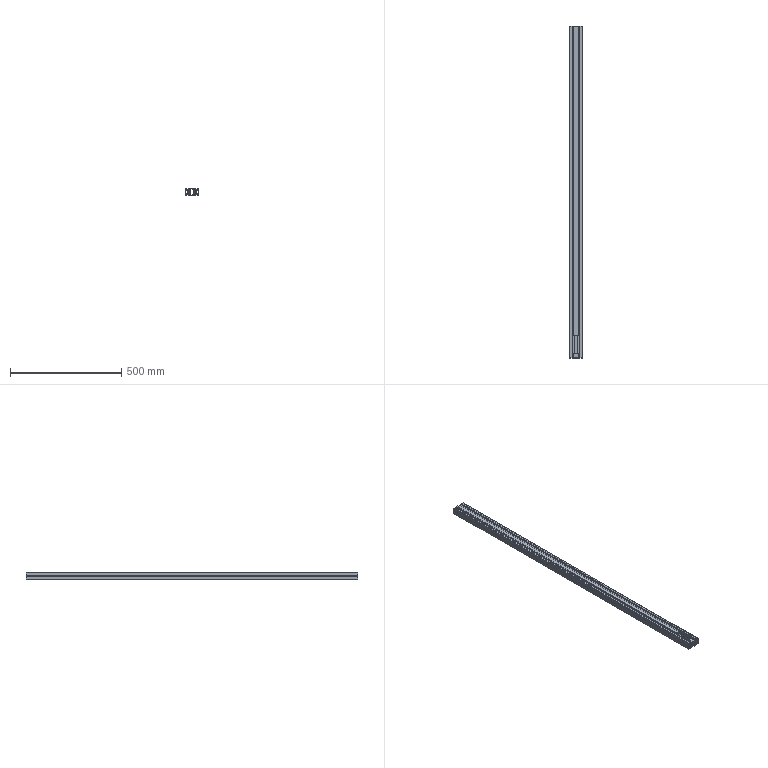Part | STEP file | 02-06 Side frame 2 | 1 solid | 106 faces | box 60 x 1495 x 30 mm | volume 1313620 mm3 | plane 80 | cylinder 26 | commonest cylinder face diameters 6 x8 5 x6 20.523 x6 2 x4 17.044 x2